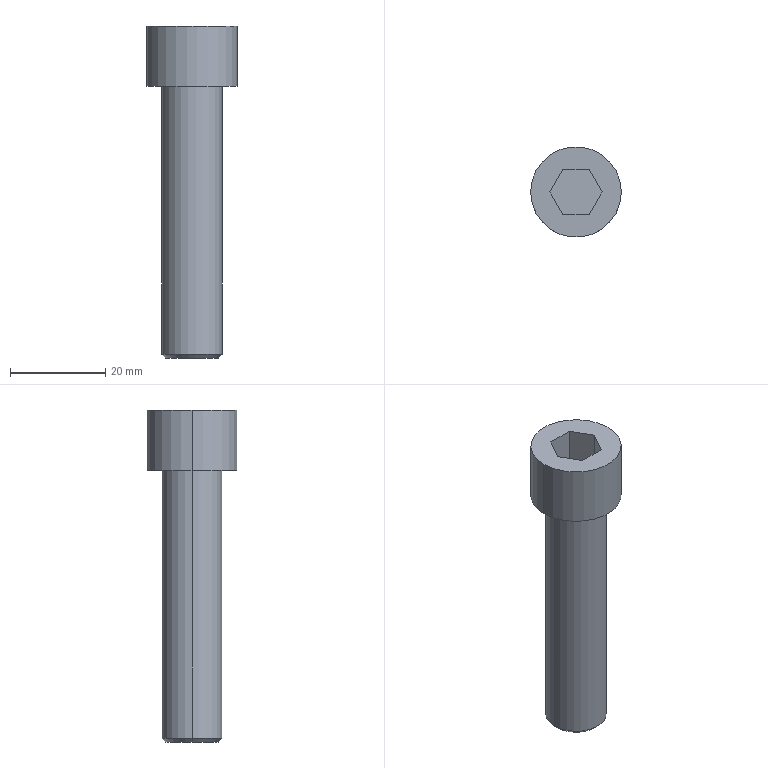Part | STEP file | 4-20.sldasm-Part-419 | 1 solid | 16 faces | box 19.05 x 19.05 x 69.85 mm | volume 10189 mm3 | plane 10 | cylinder 4 | cone 2 | commonest cylinder face diameters 12.7 x2 19.05 x2
STEP:
#1=CARTESIAN_POINT('',(-90.556,-40.,210.388));
#2=VERTEX_POINT('',#1);
#3=CARTESIAN_POINT('',(-79.444,-40.,210.388));
#4=VERTEX_POINT('',#3);
#5=CARTESIAN_POINT('',(-85.,-40.,210.388));
#6=DIRECTION('',(0.,0.,-1.));
#7=DIRECTION('',(1.,0.,0.));
#8=AXIS2_PLACEMENT_3D('',#5,#6,#7);
#9=CIRCLE('',#8,5.556);
#10=EDGE_CURVE('',#2,#4,#9,.T.);
#11=ORIENTED_EDGE('',*,*,#10,.F.);
#12=CARTESIAN_POINT('',(-91.35,-40.,211.182));
#13=VERTEX_POINT('',#12);
#14=CARTESIAN_POINT('',(-91.35,-40.,211.182));
#15=DIRECTION('',(-0.7071,0.,0.7071));
#16=VECTOR('',#15,1000.);
#17=LINE('',#14,#16);
#18=EDGE_CURVE('',#2,#13,#17,.T.);
#19=ORIENTED_EDGE('',*,*,#18,.T.);
#20=CARTESIAN_POINT('',(-78.65,-40.,211.182));
#21=VERTEX_POINT('',#20);
#22=CARTESIAN_POINT('',(-85.,-40.,211.182));
#23=DIRECTION('',(0.,0.,1.));
#24=DIRECTION('',(1.,0.,0.));
#25=AXIS2_PLACEMENT_3D('',#22,#23,#24);
#26=CIRCLE('',#25,6.35);
#27=EDGE_CURVE('',#21,#13,#26,.T.);
#28=ORIENTED_EDGE('',*,*,#27,.F.);
#29=CARTESIAN_POINT('',(-78.65,-40.,211.182));
#30=DIRECTION('',(0.7071,0.,0.7071));
#31=VECTOR('',#30,1000.);
#32=LINE('',#29,#31);
#33=EDGE_CURVE('',#4,#21,#32,.T.);
#34=ORIENTED_EDGE('',*,*,#33,.F.);
#35=EDGE_LOOP('',(#11,#19,#28,#34));
#36=FACE_OUTER_BOUND('',#35,.T.);
#37=CARTESIAN_POINT('',(-85.,-40.,211.182));
#38=DIRECTION('',(0.,0.,1.));
#39=DIRECTION('',(1.,0.,0.));
#40=AXIS2_PLACEMENT_3D('',#37,#38,#39);
#41=CONICAL_SURFACE('',#40,6.35,0.7854);
#42=ADVANCED_FACE('',(#36),#41,.T.);
#43=CARTESIAN_POINT('',(-75.475,-40.,267.538));
#44=VERTEX_POINT('',#43);
#45=CARTESIAN_POINT('',(-94.525,-40.,267.538));
#46=VERTEX_POINT('',#45);
#47=CARTESIAN_POINT('',(-85.,-40.,267.538));
#48=DIRECTION('',(0.,0.,1.));
#49=DIRECTION('',(1.,0.,0.));
#50=AXIS2_PLACEMENT_3D('',#47,#48,#49);
#51=CIRCLE('',#50,9.525);
#52=EDGE_CURVE('',#44,#46,#51,.T.);
#53=ORIENTED_EDGE('',*,*,#52,.T.);
#54=CARTESIAN_POINT('',(-94.525,-40.,280.238));
#55=VERTEX_POINT('',#54);
#56=CARTESIAN_POINT('',(-94.525,-40.,267.538));
#57=DIRECTION('',(0.,0.,1.));
#58=VECTOR('',#57,1000.);
#59=LINE('',#56,#58);
#60=EDGE_CURVE('',#46,#55,#59,.T.);
#61=ORIENTED_EDGE('',*,*,#60,.T.);
#62=CARTESIAN_POINT('',(-75.475,-40.,280.238));
#63=VERTEX_POINT('',#62);
#64=CARTESIAN_POINT('',(-85.,-40.,280.238));
#65=DIRECTION('',(0.,0.,1.));
#66=DIRECTION('',(1.,0.,0.));
#67=AXIS2_PLACEMENT_3D('',#64,#65,#66);
#68=CIRCLE('',#67,9.525);
#69=EDGE_CURVE('',#63,#55,#68,.T.);
#70=ORIENTED_EDGE('',*,*,#69,.F.);
#71=CARTESIAN_POINT('',(-75.475,-40.,267.538));
#72=DIRECTION('',(0.,0.,1.));
#73=VECTOR('',#72,1000.);
#74=LINE('',#71,#73);
#75=EDGE_CURVE('',#44,#63,#74,.T.);
#76=ORIENTED_EDGE('',*,*,#75,.F.);
#77=EDGE_LOOP('',(#53,#61,#70,#76));
#78=FACE_OUTER_BOUND('',#77,.T.);
#79=CARTESIAN_POINT('',(-85.,-40.,267.538));
#80=DIRECTION('',(0.,0.,1.));
#81=DIRECTION('',(1.,0.,0.));
#82=AXIS2_PLACEMENT_3D('',#79,#80,#81);
#83=CYLINDRICAL_SURFACE('',#82,9.525);
#84=ADVANCED_FACE('',(#78),#83,.T.);
#85=CARTESIAN_POINT('',(-78.65,-40.,267.538));
#86=VERTEX_POINT('',#85);
#87=CARTESIAN_POINT('',(-91.35,-40.,267.538));
#88=VERTEX_POINT('',#87);
#89=CARTESIAN_POINT('',(-85.,-40.,267.538));
#90=DIRECTION('',(0.,0.,1.));
#91=DIRECTION('',(1.,0.,0.));
#92=AXIS2_PLACEMENT_3D('',#89,#90,#91);
#93=CIRCLE('',#92,6.35);
#94=EDGE_CURVE('',#86,#88,#93,.T.);
#95=ORIENTED_EDGE('',*,*,#94,.F.);
#96=CARTESIAN_POINT('',(-78.65,-40.,267.538));
#97=DIRECTION('',(0.,0.,-1.));
#98=VECTOR('',#97,1000.);
#99=LINE('',#96,#98);
#100=EDGE_CURVE('',#86,#21,#99,.T.);
#101=ORIENTED_EDGE('',*,*,#100,.T.);
#102=ORIENTED_EDGE('',*,*,#27,.T.);
#103=CARTESIAN_POINT('',(-91.35,-40.,267.538));
#104=DIRECTION('',(0.,0.,-1.));
#105=VECTOR('',#104,1000.);
#106=LINE('',#103,#105);
#107=EDGE_CURVE('',#88,#13,#106,.T.);
#108=ORIENTED_EDGE('',*,*,#107,.F.);
#109=EDGE_LOOP('',(#95,#101,#102,#108));
#110=FACE_OUTER_BOUND('',#109,.T.);
#111=CARTESIAN_POINT('',(-85.,-40.,267.538));
#112=DIRECTION('',(0.,0.,-1.));
#113=DIRECTION('',(-1.,0.,0.));
#114=AXIS2_PLACEMENT_3D('',#111,#112,#113);
#115=CYLINDRICAL_SURFACE('',#114,6.35);
#116=ADVANCED_FACE('',(#110),#115,.T.);
#117=ORIENTED_EDGE('',*,*,#100,.F.);
#118=CARTESIAN_POINT('',(-85.,-40.,267.538));
#119=DIRECTION('',(0.,0.,1.));
#120=DIRECTION('',(1.,0.,0.));
#121=AXIS2_PLACEMENT_3D('',#118,#119,#120);
#122=CIRCLE('',#121,6.35);
#123=EDGE_CURVE('',#88,#86,#122,.T.);
#124=ORIENTED_EDGE('',*,*,#123,.F.);
#125=ORIENTED_EDGE('',*,*,#107,.T.);
#126=CARTESIAN_POINT('',(-85.,-40.,211.182));
#127=DIRECTION('',(0.,0.,1.));
#128=DIRECTION('',(1.,0.,0.));
#129=AXIS2_PLACEMENT_3D('',#126,#127,#128);
#130=CIRCLE('',#129,6.35);
#131=EDGE_CURVE('',#13,#21,#130,.T.);
#132=ORIENTED_EDGE('',*,*,#131,.T.);
#133=EDGE_LOOP('',(#117,#124,#125,#132));
#134=FACE_OUTER_BOUND('',#133,.T.);
#135=CARTESIAN_POINT('',(-85.,-40.,267.538));
#136=DIRECTION('',(0.,0.,-1.));
#137=DIRECTION('',(-1.,0.,0.));
#138=AXIS2_PLACEMENT_3D('',#135,#136,#137);
#139=CYLINDRICAL_SURFACE('',#138,6.35);
#140=ADVANCED_FACE('',(#134),#139,.T.);
#141=CARTESIAN_POINT('',(-85.,-40.,210.388));
#142=DIRECTION('',(0.,0.,-1.));
#143=DIRECTION('',(1.,0.,0.));
#144=AXIS2_PLACEMENT_3D('',#141,#142,#143);
#145=CIRCLE('',#144,5.556);
#146=EDGE_CURVE('',#4,#2,#145,.T.);
#147=ORIENTED_EDGE('',*,*,#146,.T.);
#148=ORIENTED_EDGE('',*,*,#10,.T.);
#149=EDGE_LOOP('',(#147,#148));
#150=FACE_OUTER_BOUND('',#149,.T.);
#151=CARTESIAN_POINT('',(-85.,-40.,210.388));
#152=DIRECTION('',(0.,0.,1.));
#153=DIRECTION('',(1.,0.,0.));
#154=AXIS2_PLACEMENT_3D('',#151,#152,#153);
#155=PLANE('',#154);
#156=ADVANCED_FACE('',(#150),#155,.F.);
#157=ORIENTED_EDGE('',*,*,#52,.F.);
#158=CARTESIAN_POINT('',(-85.,-40.,267.538));
#159=DIRECTION('',(0.,0.,1.));
#160=DIRECTION('',(1.,0.,0.));
#161=AXIS2_PLACEMENT_3D('',#158,#159,#160);
#162=CIRCLE('',#161,9.525);
#163=EDGE_CURVE('',#46,#44,#162,.T.);
#164=ORIENTED_EDGE('',*,*,#163,.F.);
#165=EDGE_LOOP('',(#157,#164));
#166=FACE_OUTER_BOUND('',#165,.T.);
#167=ORIENTED_EDGE('',*,*,#123,.T.);
#168=ORIENTED_EDGE('',*,*,#94,.T.);
#169=EDGE_LOOP('',(#167,#168));
#170=FACE_BOUND('',#169,.T.);
#171=CARTESIAN_POINT('',(-85.,-40.,267.538));
#172=DIRECTION('',(0.,0.,-1.));
#173=DIRECTION('',(-1.,0.,0.));
#174=AXIS2_PLACEMENT_3D('',#171,#172,#173);
#175=PLANE('',#174);
#176=ADVANCED_FACE('',(#166,#170),#175,.T.);
#177=CARTESIAN_POINT('',(-87.75,-44.763,280.238));
#178=VERTEX_POINT('',#177);
#179=CARTESIAN_POINT('',(-82.25,-44.763,280.238));
#180=VERTEX_POINT('',#179);
#181=CARTESIAN_POINT('',(-87.75,-44.763,280.238));
#182=DIRECTION('',(1.,0.,0.));
#183=VECTOR('',#182,1000.);
#184=LINE('',#181,#183);
#185=EDGE_CURVE('',#178,#180,#184,.T.);
#186=ORIENTED_EDGE('',*,*,#185,.F.);
#187=CARTESIAN_POINT('',(-90.499,-40.,280.238));
#188=VERTEX_POINT('',#187);
#189=CARTESIAN_POINT('',(-90.499,-40.,280.238));
#190=DIRECTION('',(0.5,-0.866,0.));
#191=VECTOR('',#190,1000.);
#192=LINE('',#189,#191);
#193=EDGE_CURVE('',#188,#178,#192,.T.);
#194=ORIENTED_EDGE('',*,*,#193,.F.);
#195=CARTESIAN_POINT('',(-87.75,-35.238,280.238));
#196=VERTEX_POINT('',#195);
#197=CARTESIAN_POINT('',(-87.75,-35.238,280.238));
#198=DIRECTION('',(-0.5,-0.866,0.));
#199=VECTOR('',#198,1000.);
#200=LINE('',#197,#199);
#201=EDGE_CURVE('',#196,#188,#200,.T.);
#202=ORIENTED_EDGE('',*,*,#201,.F.);
#203=CARTESIAN_POINT('',(-82.25,-35.238,280.238));
#204=VERTEX_POINT('',#203);
#205=CARTESIAN_POINT('',(-82.25,-35.238,280.238));
#206=DIRECTION('',(-1.,0.,0.));
#207=VECTOR('',#206,1000.);
#208=LINE('',#205,#207);
#209=EDGE_CURVE('',#204,#196,#208,.T.);
#210=ORIENTED_EDGE('',*,*,#209,.F.);
#211=CARTESIAN_POINT('',(-79.501,-40.,280.238));
#212=VERTEX_POINT('',#211);
#213=CARTESIAN_POINT('',(-79.501,-40.,280.238));
#214=DIRECTION('',(-0.5,0.866,0.));
#215=VECTOR('',#214,1000.);
#216=LINE('',#213,#215);
#217=EDGE_CURVE('',#212,#204,#216,.T.);
#218=ORIENTED_EDGE('',*,*,#217,.F.);
#219=CARTESIAN_POINT('',(-82.25,-44.763,280.238));
#220=DIRECTION('',(0.5,0.866,0.));
#221=VECTOR('',#220,1000.);
#222=LINE('',#219,#221);
#223=EDGE_CURVE('',#180,#212,#222,.T.);
#224=ORIENTED_EDGE('',*,*,#223,.F.);
#225=EDGE_LOOP('',(#186,#194,#202,#210,#218,#224));
#226=FACE_BOUND('',#225,.T.);
#227=ORIENTED_EDGE('',*,*,#69,.T.);
#228=CARTESIAN_POINT('',(-85.,-40.,280.238));
#229=DIRECTION('',(0.,0.,1.));
#230=DIRECTION('',(1.,0.,0.));
#231=AXIS2_PLACEMENT_3D('',#228,#229,#230);
#232=CIRCLE('',#231,9.525);
#233=EDGE_CURVE('',#55,#63,#232,.T.);
#234=ORIENTED_EDGE('',*,*,#233,.T.);
#235=EDGE_LOOP('',(#227,#234));
#236=FACE_OUTER_BOUND('',#235,.T.);
#237=CARTESIAN_POINT('',(-85.,-40.,280.238));
#238=DIRECTION('',(0.,0.,1.));
#239=DIRECTION('',(1.,0.,0.));
#240=AXIS2_PLACEMENT_3D('',#237,#238,#239);
#241=PLANE('',#240);
#242=ADVANCED_FACE('',(#226,#236),#241,.T.);
#243=ORIENTED_EDGE('',*,*,#60,.F.);
#244=ORIENTED_EDGE('',*,*,#163,.T.);
#245=ORIENTED_EDGE('',*,*,#75,.T.);
#246=ORIENTED_EDGE('',*,*,#233,.F.);
#247=EDGE_LOOP('',(#243,#244,#245,#246));
#248=FACE_OUTER_BOUND('',#247,.T.);
#249=CARTESIAN_POINT('',(-85.,-40.,267.538));
#250=DIRECTION('',(0.,0.,1.));
#251=DIRECTION('',(1.,0.,0.));
#252=AXIS2_PLACEMENT_3D('',#249,#250,#251);
#253=CYLINDRICAL_SURFACE('',#252,9.525);
#254=ADVANCED_FACE('',(#248),#253,.T.);
#255=ORIENTED_EDGE('',*,*,#18,.F.);
#256=ORIENTED_EDGE('',*,*,#146,.F.);
#257=ORIENTED_EDGE('',*,*,#33,.T.);
#258=ORIENTED_EDGE('',*,*,#131,.F.);
#259=EDGE_LOOP('',(#255,#256,#257,#258));
#260=FACE_OUTER_BOUND('',#259,.T.);
#261=CARTESIAN_POINT('',(-85.,-40.,211.182));
#262=DIRECTION('',(0.,0.,1.));
#263=DIRECTION('',(1.,0.,0.));
#264=AXIS2_PLACEMENT_3D('',#261,#262,#263);
#265=CONICAL_SURFACE('',#264,6.35,0.7854);
#266=ADVANCED_FACE('',(#260),#265,.T.);
#267=ORIENTED_EDGE('',*,*,#185,.T.);
#268=CARTESIAN_POINT('',(-82.25,-44.763,271.856));
#269=VERTEX_POINT('',#268);
#270=CARTESIAN_POINT('',(-82.25,-44.763,271.856));
#271=DIRECTION('',(0.,0.,1.));
#272=VECTOR('',#271,1000.);
#273=LINE('',#270,#272);
#274=EDGE_CURVE('',#269,#180,#273,.T.);
#275=ORIENTED_EDGE('',*,*,#274,.F.);
#276=CARTESIAN_POINT('',(-87.75,-44.763,271.856));
#277=VERTEX_POINT('',#276);
#278=CARTESIAN_POINT('',(-87.75,-44.763,271.856));
#279=DIRECTION('',(1.,0.,0.));
#280=VECTOR('',#279,1000.);
#281=LINE('',#278,#280);
#282=EDGE_CURVE('',#277,#269,#281,.T.);
#283=ORIENTED_EDGE('',*,*,#282,.F.);
#284=CARTESIAN_POINT('',(-87.75,-44.763,271.856));
#285=DIRECTION('',(0.,0.,1.));
#286=VECTOR('',#285,1000.);
#287=LINE('',#284,#286);
#288=EDGE_CURVE('',#277,#178,#287,.T.);
#289=ORIENTED_EDGE('',*,*,#288,.T.);
#290=EDGE_LOOP('',(#267,#275,#283,#289));
#291=FACE_OUTER_BOUND('',#290,.T.);
#292=CARTESIAN_POINT('',(-87.75,-44.763,271.856));
#293=DIRECTION('',(0.,-1.,0.));
#294=DIRECTION('',(0.,0.,-1.));
#295=AXIS2_PLACEMENT_3D('',#292,#293,#294);
#296=PLANE('',#295);
#297=ADVANCED_FACE('',(#291),#296,.F.);
#298=ORIENTED_EDGE('',*,*,#223,.T.);
#299=CARTESIAN_POINT('',(-79.501,-40.,271.856));
#300=VERTEX_POINT('',#299);
#301=CARTESIAN_POINT('',(-79.501,-40.,271.856));
#302=DIRECTION('',(0.,0.,1.));
#303=VECTOR('',#302,1000.);
#304=LINE('',#301,#303);
#305=EDGE_CURVE('',#300,#212,#304,.T.);
#306=ORIENTED_EDGE('',*,*,#305,.F.);
#307=CARTESIAN_POINT('',(-82.25,-44.763,271.856));
#308=DIRECTION('',(0.5,0.866,0.));
#309=VECTOR('',#308,1000.);
#310=LINE('',#307,#309);
#311=EDGE_CURVE('',#269,#300,#310,.T.);
#312=ORIENTED_EDGE('',*,*,#311,.F.);
#313=ORIENTED_EDGE('',*,*,#274,.T.);
#314=EDGE_LOOP('',(#298,#306,#312,#313));
#315=FACE_OUTER_BOUND('',#314,.T.);
#316=CARTESIAN_POINT('',(-82.25,-44.763,271.856));
#317=DIRECTION('',(0.866,-0.5,0.));
#318=DIRECTION('',(0.5,0.866,0.));
#319=AXIS2_PLACEMENT_3D('',#316,#317,#318);
#320=PLANE('',#319);
#321=ADVANCED_FACE('',(#315),#320,.F.);
#322=ORIENTED_EDGE('',*,*,#217,.T.);
#323=CARTESIAN_POINT('',(-82.25,-35.238,271.856));
#324=VERTEX_POINT('',#323);
#325=CARTESIAN_POINT('',(-82.25,-35.238,271.856));
#326=DIRECTION('',(0.,0.,1.));
#327=VECTOR('',#326,1000.);
#328=LINE('',#325,#327);
#329=EDGE_CURVE('',#324,#204,#328,.T.);
#330=ORIENTED_EDGE('',*,*,#329,.F.);
#331=CARTESIAN_POINT('',(-79.501,-40.,271.856));
#332=DIRECTION('',(-0.5,0.866,0.));
#333=VECTOR('',#332,1000.);
#334=LINE('',#331,#333);
#335=EDGE_CURVE('',#300,#324,#334,.T.);
#336=ORIENTED_EDGE('',*,*,#335,.F.);
#337=ORIENTED_EDGE('',*,*,#305,.T.);
#338=EDGE_LOOP('',(#322,#330,#336,#337));
#339=FACE_OUTER_BOUND('',#338,.T.);
#340=CARTESIAN_POINT('',(-79.501,-40.,271.856));
#341=DIRECTION('',(0.866,0.5,0.));
#342=DIRECTION('',(-0.5,0.866,0.));
#343=AXIS2_PLACEMENT_3D('',#340,#341,#342);
#344=PLANE('',#343);
#345=ADVANCED_FACE('',(#339),#344,.F.);
#346=ORIENTED_EDGE('',*,*,#209,.T.);
#347=CARTESIAN_POINT('',(-87.75,-35.238,271.856));
#348=VERTEX_POINT('',#347);
#349=CARTESIAN_POINT('',(-87.75,-35.238,271.856));
#350=DIRECTION('',(0.,0.,1.));
#351=VECTOR('',#350,1000.);
#352=LINE('',#349,#351);
#353=EDGE_CURVE('',#348,#196,#352,.T.);
#354=ORIENTED_EDGE('',*,*,#353,.F.);
#355=CARTESIAN_POINT('',(-82.25,-35.238,271.856));
#356=DIRECTION('',(-1.,0.,0.));
#357=VECTOR('',#356,1000.);
#358=LINE('',#355,#357);
#359=EDGE_CURVE('',#324,#348,#358,.T.);
#360=ORIENTED_EDGE('',*,*,#359,.F.);
#361=ORIENTED_EDGE('',*,*,#329,.T.);
#362=EDGE_LOOP('',(#346,#354,#360,#361));
#363=FACE_OUTER_BOUND('',#362,.T.);
#364=CARTESIAN_POINT('',(-82.25,-35.238,271.856));
#365=DIRECTION('',(0.,1.,0.));
#366=DIRECTION('',(0.,0.,1.));
#367=AXIS2_PLACEMENT_3D('',#364,#365,#366);
#368=PLANE('',#367);
#369=ADVANCED_FACE('',(#363),#368,.F.);
#370=ORIENTED_EDGE('',*,*,#201,.T.);
#371=CARTESIAN_POINT('',(-90.499,-40.,271.856));
#372=VERTEX_POINT('',#371);
#373=CARTESIAN_POINT('',(-90.499,-40.,271.856));
#374=DIRECTION('',(0.,0.,1.));
#375=VECTOR('',#374,1000.);
#376=LINE('',#373,#375);
#377=EDGE_CURVE('',#372,#188,#376,.T.);
#378=ORIENTED_EDGE('',*,*,#377,.F.);
#379=CARTESIAN_POINT('',(-87.75,-35.238,271.856));
#380=DIRECTION('',(-0.5,-0.866,0.));
#381=VECTOR('',#380,1000.);
#382=LINE('',#379,#381);
#383=EDGE_CURVE('',#348,#372,#382,.T.);
#384=ORIENTED_EDGE('',*,*,#383,.F.);
#385=ORIENTED_EDGE('',*,*,#353,.T.);
#386=EDGE_LOOP('',(#370,#378,#384,#385));
#387=FACE_OUTER_BOUND('',#386,.T.);
#388=CARTESIAN_POINT('',(-87.75,-35.238,271.856));
#389=DIRECTION('',(-0.866,0.5,0.));
#390=DIRECTION('',(-0.5,-0.866,0.));
#391=AXIS2_PLACEMENT_3D('',#388,#389,#390);
#392=PLANE('',#391);
#393=ADVANCED_FACE('',(#387),#392,.F.);
#394=ORIENTED_EDGE('',*,*,#193,.T.);
#395=ORIENTED_EDGE('',*,*,#288,.F.);
#396=CARTESIAN_POINT('',(-90.499,-40.,271.856));
#397=DIRECTION('',(0.5,-0.866,0.));
#398=VECTOR('',#397,1000.);
#399=LINE('',#396,#398);
#400=EDGE_CURVE('',#372,#277,#399,.T.);
#401=ORIENTED_EDGE('',*,*,#400,.F.);
#402=ORIENTED_EDGE('',*,*,#377,.T.);
#403=EDGE_LOOP('',(#394,#395,#401,#402));
#404=FACE_OUTER_BOUND('',#403,.T.);
#405=CARTESIAN_POINT('',(-90.499,-40.,271.856));
#406=DIRECTION('',(-0.866,-0.5,0.));
#407=DIRECTION('',(0.5,-0.866,0.));
#408=AXIS2_PLACEMENT_3D('',#405,#406,#407);
#409=PLANE('',#408);
#410=ADVANCED_FACE('',(#404),#409,.F.);
#411=ORIENTED_EDGE('',*,*,#282,.T.);
#412=ORIENTED_EDGE('',*,*,#311,.T.);
#413=ORIENTED_EDGE('',*,*,#335,.T.);
#414=ORIENTED_EDGE('',*,*,#359,.T.);
#415=ORIENTED_EDGE('',*,*,#383,.T.);
#416=ORIENTED_EDGE('',*,*,#400,.T.);
#417=EDGE_LOOP('',(#411,#412,#413,#414,#415,#416));
#418=FACE_OUTER_BOUND('',#417,.T.);
#419=CARTESIAN_POINT('',(-82.25,-44.763,271.856));
#420=DIRECTION('',(0.,0.,1.));
#421=DIRECTION('',(1.,0.,0.));
#422=AXIS2_PLACEMENT_3D('',#419,#420,#421);
#423=PLANE('',#422);
#424=ADVANCED_FACE('',(#418),#423,.T.);
#425=CLOSED_SHELL('',(#42,#84,#116,#140,#156,#176,#242,#254,#266,#297,#321,#345,#369,#393,#410,#424));
#426=MANIFOLD_SOLID_BREP('',#425);
#427=CARTESIAN_POINT('',(0.,0.,0.));
#428=DIRECTION('',(0.,0.,1.));
#429=DIRECTION('',(1.,0.,0.));
#430=AXIS2_PLACEMENT_3D('',#427,#428,#429);
#431=(LENGTH_UNIT()NAMED_UNIT(*)SI_UNIT(.MILLI.,.METRE.));
#432=UNCERTAINTY_MEASURE_WITH_UNIT(LENGTH_MEASURE(0.00001),#431,'','');
#433=(NAMED_UNIT(*)PLANE_ANGLE_UNIT()SI_UNIT($,.RADIAN.));
#434=(NAMED_UNIT(*)SI_UNIT($,.STERADIAN.)SOLID_ANGLE_UNIT());
#435=(GEOMETRIC_REPRESENTATION_CONTEXT(3)GLOBAL_UNCERTAINTY_ASSIGNED_CONTEXT((#432))GLOBAL_UNIT_ASSIGNED_CONTEXT((#431,#433,#434))REPRESENTATION_CONTEXT('',''));
#436=ADVANCED_BREP_SHAPE_REPRESENTATION('',(#426,#430),#435);